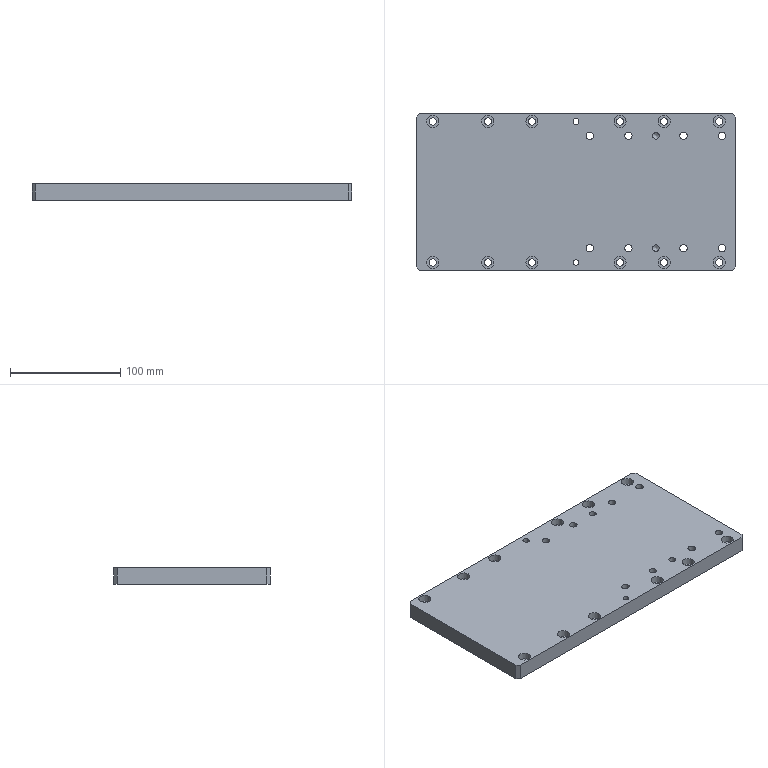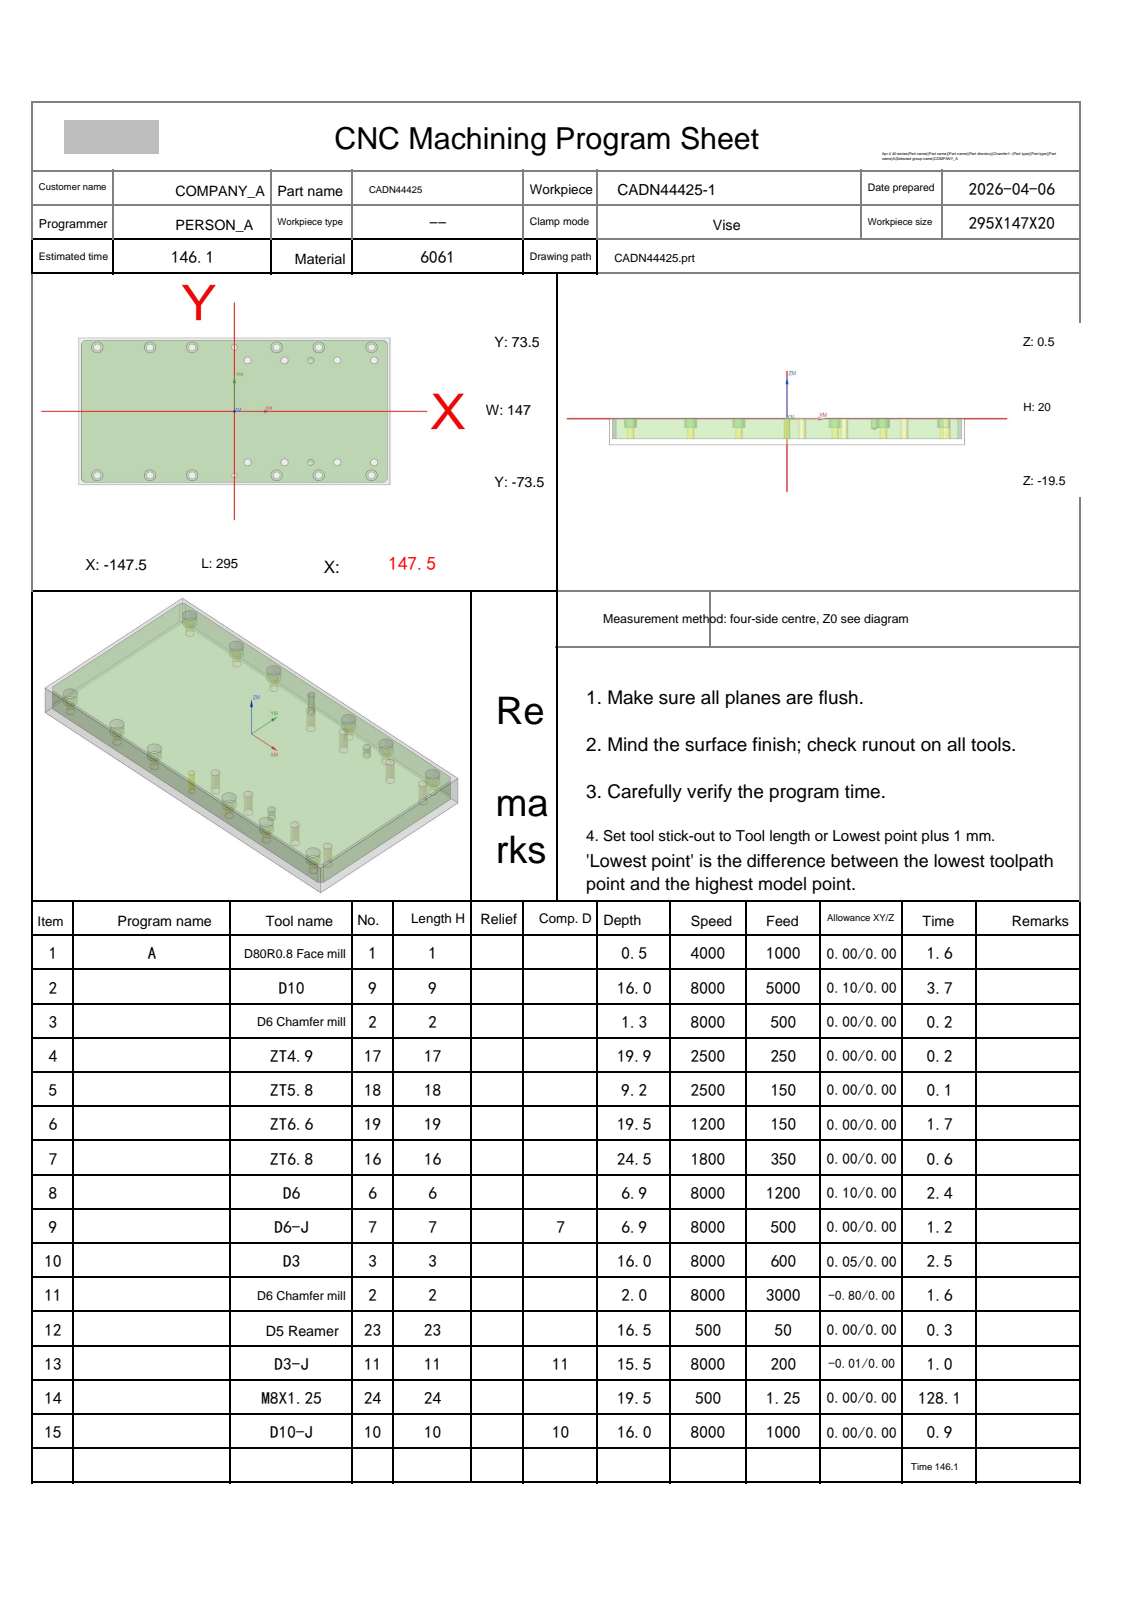NC program | NX | posted by the shop | part box 290 x 142 x 15 mm
Lines 1802 to 2582 of 2582:
N11 T02 M06
(D6 Chamfer mill  D=6. R=0. H=02 ce=0.00 di=0.00)
G00 G90 G54 X.25 Y-73.128 M03 S8000
G43 H02 Z20.
M08
Z2.099
G01 Z-1.5 F3000.
G03 X.33 Y-72.828 I-.52 J.3
X.03 Y-72.308 I-.6 J0.0
G01 X0.0 Y-72.3
X-142.
X-142.254 Y-72.275
X-142.497 Y-72.201
X-142.722 Y-72.081
X-142.919 Y-71.919
X-145.919 Y-68.919
X-146.081 Y-68.722
X-146.201 Y-68.497
X-146.275 Y-68.254
X-146.3 Y-68.
Y68.
X-146.275 Y68.254
X-146.201 Y68.497
X-146.081 Y68.722
X-145.919 Y68.919
X-142.919 Y71.919
X-142.722 Y72.081
X-142.497 Y72.201
X-142.254 Y72.275
X-142. Y72.3
X142.
X142.254 Y72.275
X142.497 Y72.201
X142.722 Y72.081
X142.919 Y71.919
X145.919 Y68.919
X146.081 Y68.722
X146.201 Y68.497
X146.275 Y68.254
X146.3 Y68.
Y-68.
X146.275 Y-68.254
X146.201 Y-68.497
X146.081 Y-68.722
X145.919 Y-68.919
X142.919 Y-71.919
X142.722 Y-72.081
X142.497 Y-72.201
X142.254 Y-72.275
X142. Y-72.3
X0.0
X-.03 Y-72.308
G03 X-.33 Y-72.828 I.3 J-.52
X-.25 Y-73.128 I.6 J0.0
G01 Z2.099
G00 Z20.
X-.372 Y64.25
Z2.099
G01 Z-1.5
G03 X-.672 Y64.33 I-.3 J-.52
X-1.192 Y64.03 I0.0 J-.6
G01 X-1.2 Y64.
Y63.5
G03 X0.0 Y62.3 I1.2 J0.0
X1.2 Y63.5 I0.0 J1.2
G01 Y64.5
G03 X0.0 Y65.7 I-1.2 J0.0
X-1.2 Y64.5 I0.0 J-1.2
G01 Y64.
X-1.192 Y63.97
G03 X-.672 Y63.67 I.52 J.3
X-.372 Y63.75 I0.0 J.6
G01 Z2.099
G00 Z20.
G00 G90 X-.157 Y-63.216 M03 S8000
Z20.
Z-.5
G01 Z-1. F500.
X-.3 Y-62.5
G03 X-1.8 Y-64. I0.0 J-1.5
X0.0 Y-65.8 I1.8 J0.0
X1.8 Y-64. I0.0 J1.8
X0.0 Y-62.2 I-1.8 J0.0
X-1.8 Y-64. I0.0 J-1.8
X-.3 Y-65.5 I1.5 J0.0
G01 X-.157 Y-64.784
Z-.5
G00 Z20.
G00 G90 X71.888 Y52.147 M03 S8000
Z20.
Z-.5
G01 Z-1. F500.
X71.7 Y52.5
G03 X70.2 Y51. I0.0 J-1.5
X72.5 Y48.7 I2.3 J0.0
X74.8 Y51. I0.0 J2.3
X72.5 Y53.3 I-2.3 J0.0
X70.2 Y51. I0.0 J-2.3
X71.7 Y49.5 I1.5 J0.0
G01 X71.888 Y49.853
Z-.5
G00 Z20.
Y-49.853
Z-.5
G01 Z-1.
X71.7 Y-49.5
G03 X70.2 Y-51. I0.0 J-1.5
X72.5 Y-53.3 I2.3 J0.0
X74.8 Y-51. I0.0 J2.3
X72.5 Y-48.7 I-2.3 J0.0
X70.2 Y-51. I0.0 J-2.3
X71.7 Y-52.5 I1.5 J0.0
G01 X71.888 Y-52.147
Z-.5
G00 Z20.
G00 G90 X131.334 Y52.5 M03 S8000
Z20.
Z-.8
G01 Z-1.3 F600.
X131.1
G03 X129.6 Y51. I0.0 J-1.5
X132.5 Y48.1 I2.9 J0.0
X135.4 Y51. I0.0 J2.9
X132.5 Y53.9 I-2.9 J0.0
X129.6 Y51. I0.0 J-2.9
X131.1 Y49.5 I1.5 J0.0
G01 X131.334
Z-.8
G00 Z20.
X96.334 Y52.5
Z-.8
G01 Z-1.3
X96.1
G03 X94.6 Y51. I0.0 J-1.5
X97.5 Y48.1 I2.9 J0.0
X100.4 Y51. I0.0 J2.9
X97.5 Y53.9 I-2.9 J0.0
X94.6 Y51. I0.0 J-2.9
X96.1 Y49.5 I1.5 J0.0
G01 X96.334
Z-.8
G00 Z20.
X46.334 Y52.5
Z-.8
G01 Z-1.3
X46.1
G03 X44.6 Y51. I0.0 J-1.5
X47.5 Y48.1 I2.9 J0.0
X50.4 Y51. I0.0 J2.9
X47.5 Y53.9 I-2.9 J0.0
X44.6 Y51. I0.0 J-2.9
X46.1 Y49.5 I1.5 J0.0
G01 X46.334
Z-.8
G00 Z20.
X11.334 Y52.5
Z-.8
G01 Z-1.3
X11.1
G03 X9.6 Y51. I0.0 J-1.5
X12.5 Y48.1 I2.9 J0.0
X15.4 Y51. I0.0 J2.9
X12.5 Y53.9 I-2.9 J0.0
X9.6 Y51. I0.0 J-2.9
X11.1 Y49.5 I1.5 J0.0
G01 X11.334
Z-.8
G00 Z20.
Y-49.5
Z-.8
G01 Z-1.3
X11.1
G03 X9.6 Y-51. I0.0 J-1.5
X12.5 Y-53.9 I2.9 J0.0
X15.4 Y-51. I0.0 J2.9
X12.5 Y-48.1 I-2.9 J0.0
X9.6 Y-51. I0.0 J-2.9
X11.1 Y-52.5 I1.5 J0.0
G01 X11.334
Z-.8
G00 Z20.
X46.334 Y-49.5
Z-.8
G01 Z-1.3
X46.1
G03 X44.6 Y-51. I0.0 J-1.5
X47.5 Y-53.9 I2.9 J0.0
X50.4 Y-51. I0.0 J2.9
X47.5 Y-48.1 I-2.9 J0.0
X44.6 Y-51. I0.0 J-2.9
X46.1 Y-52.5 I1.5 J0.0
G01 X46.334
Z-.8
G00 Z20.
X96.334 Y-49.5
Z-.8
G01 Z-1.3
X96.1
G03 X94.6 Y-51. I0.0 J-1.5
X97.5 Y-53.9 I2.9 J0.0
X100.4 Y-51. I0.0 J2.9
X97.5 Y-48.1 I-2.9 J0.0
X94.6 Y-51. I0.0 J-2.9
X96.1 Y-52.5 I1.5 J0.0
G01 X96.334
Z-.8
G00 Z20.
X131.334 Y-49.5
Z-.8
G01 Z-1.3
X131.1
G03 X129.6 Y-51. I0.0 J-1.5
X132.5 Y-53.9 I2.9 J0.0
X135.4 Y-51. I0.0 J2.9
X132.5 Y-48.1 I-2.9 J0.0
X129.6 Y-51. I0.0 J-2.9
X131.1 Y-52.5 I1.5 J0.0
G01 X131.334
Z-.8
G00 Z20.
G00 G90 X127.991 Y-68.357 M03 S8000
Z20.
Z2.5
G01 X128.166 Y-68.439 Z2.43 F800.
X128.601 Y-68.595 Z2.261
X129.05 Y-68.708 Z2.093
X129.507 Y-68.778 Z1.925
X129.969 Y-68.803 Z1.756
X130.431 Y-68.784 Z1.588
X130.89 Y-68.72 Z1.419
X131.34 Y-68.612 Z1.251
X131.777 Y-68.462 Z1.083
X132.198 Y-68.27 Z.914
X132.599 Y-68.039 Z.746
X132.976 Y-67.77 Z.577
X133.325 Y-67.466 Z.409
X133.643 Y-67.13 Z.241
X133.927 Y-66.765 Z.072
X134.175 Y-66.375 Z-.096
X134.384 Y-65.962 Z-.265
X134.552 Y-65.531 Z-.433
X134.679 Y-65.086 Z-.601
X134.761 Y-64.631 Z-.77
X134.8 Y-64.17 Z-.938
Y-64. Z-1.
G03 X130. Y-59.2 I-4.8 J0.0
X125.2 Y-64. I0.0 J-4.8
X130. Y-68.8 I4.8 J0.0
X134.8 Y-64. I0.0 J4.8
X134.774 Y-63.501 I-4.8 J0.0
G01 Z1.5
G00 Z20.
X77.991 Y-68.357
Z2.5
G01 X78.166 Y-68.439 Z2.43
X78.601 Y-68.595 Z2.261
X79.05 Y-68.708 Z2.093
X79.507 Y-68.778 Z1.925
X79.969 Y-68.803 Z1.756
X80.431 Y-68.784 Z1.588
X80.89 Y-68.72 Z1.419
X81.34 Y-68.612 Z1.251
X81.777 Y-68.462 Z1.083
X82.198 Y-68.27 Z.914
X82.599 Y-68.039 Z.746
X82.976 Y-67.77 Z.577
X83.325 Y-67.466 Z.409
X83.643 Y-67.13 Z.241
X83.927 Y-66.765 Z.072
X84.175 Y-66.375 Z-.096
X84.384 Y-65.962 Z-.265
X84.552 Y-65.531 Z-.433
X84.679 Y-65.086 Z-.601
X84.761 Y-64.631 Z-.77
X84.8 Y-64.17 Z-.938
Y-64. Z-1.
G03 X80. Y-59.2 I-4.8 J0.0
X75.2 Y-64. I0.0 J-4.8
X80. Y-68.8 I4.8 J0.0
X84.8 Y-64. I0.0 J4.8
X84.774 Y-63.501 I-4.8 J0.0
G01 Z1.5
G00 Z20.
X37.991 Y-68.357
Z2.5
G01 X38.166 Y-68.439 Z2.43
X38.601 Y-68.595 Z2.261
X39.05 Y-68.708 Z2.093
X39.507 Y-68.778 Z1.925
X39.969 Y-68.803 Z1.756
X40.431 Y-68.784 Z1.588
X40.89 Y-68.72 Z1.419
X41.34 Y-68.612 Z1.251
X41.777 Y-68.462 Z1.083
X42.198 Y-68.27 Z.914
X42.599 Y-68.039 Z.746
X42.976 Y-67.77 Z.577
X43.325 Y-67.466 Z.409
X43.643 Y-67.13 Z.241
X43.927 Y-66.765 Z.072
X44.175 Y-66.375 Z-.096
X44.384 Y-65.962 Z-.265
X44.552 Y-65.531 Z-.433
X44.679 Y-65.086 Z-.601
X44.761 Y-64.631 Z-.77
X44.8 Y-64.17 Z-.938
Y-64. Z-1.
G03 X40. Y-59.2 I-4.8 J0.0
X35.2 Y-64. I0.0 J-4.8
X40. Y-68.8 I4.8 J0.0
X44.8 Y-64. I0.0 J4.8
X44.774 Y-63.501 I-4.8 J0.0
G01 Z1.5
G00 Z20.
X-42.009 Y-68.357
Z2.5
G01 X-41.834 Y-68.439 Z2.43
X-41.399 Y-68.595 Z2.261
X-40.95 Y-68.708 Z2.093
X-40.493 Y-68.778 Z1.925
X-40.031 Y-68.803 Z1.756
X-39.569 Y-68.784 Z1.588
X-39.11 Y-68.72 Z1.419
X-38.66 Y-68.612 Z1.251
X-38.223 Y-68.462 Z1.083
X-37.802 Y-68.27 Z.914
X-37.401 Y-68.039 Z.746
X-37.024 Y-67.77 Z.577
X-36.675 Y-67.466 Z.409
X-36.357 Y-67.13 Z.241
X-36.073 Y-66.765 Z.072
X-35.825 Y-66.375 Z-.096
X-35.616 Y-65.962 Z-.265
X-35.448 Y-65.531 Z-.433
X-35.321 Y-65.086 Z-.601
X-35.239 Y-64.631 Z-.77
X-35.2 Y-64.17 Z-.938
Y-64. Z-1.
G03 X-40. Y-59.2 I-4.8 J0.0
X-44.8 Y-64. I0.0 J-4.8
X-40. Y-68.8 I4.8 J0.0
X-35.2 Y-64. I0.0 J4.8
X-35.226 Y-63.501 I-4.8 J0.0
G01 Z1.5
G00 Z20.
X-82.009 Y-68.357
Z2.5
G01 X-81.834 Y-68.439 Z2.43
X-81.399 Y-68.595 Z2.261
X-80.95 Y-68.708 Z2.093
X-80.493 Y-68.778 Z1.925
X-80.031 Y-68.803 Z1.756
X-79.569 Y-68.784 Z1.588
X-79.11 Y-68.72 Z1.419
X-78.66 Y-68.612 Z1.251
X-78.223 Y-68.462 Z1.083
X-77.802 Y-68.27 Z.914
X-77.401 Y-68.039 Z.746
X-77.024 Y-67.77 Z.577
X-76.675 Y-67.466 Z.409
X-76.357 Y-67.13 Z.241
X-76.073 Y-66.765 Z.072
X-75.825 Y-66.375 Z-.096
X-75.616 Y-65.962 Z-.265
X-75.448 Y-65.531 Z-.433
X-75.321 Y-65.086 Z-.601
X-75.239 Y-64.631 Z-.77
X-75.2 Y-64.17 Z-.938
Y-64. Z-1.
G03 X-80. Y-59.2 I-4.8 J0.0
X-84.8 Y-64. I0.0 J-4.8
X-80. Y-68.8 I4.8 J0.0
X-75.2 Y-64. I0.0 J4.8
X-75.226 Y-63.501 I-4.8 J0.0
G01 Z1.5
G00 Z20.
X-132.009 Y-68.357
Z2.5
G01 X-131.834 Y-68.439 Z2.43
X-131.399 Y-68.595 Z2.261
X-130.95 Y-68.708 Z2.093
X-130.493 Y-68.778 Z1.925
X-130.031 Y-68.803 Z1.756
X-129.569 Y-68.784 Z1.588
X-129.11 Y-68.72 Z1.419
X-128.66 Y-68.612 Z1.251
X-128.223 Y-68.462 Z1.083
X-127.802 Y-68.27 Z.914
X-127.401 Y-68.039 Z.746
X-127.024 Y-67.77 Z.577
X-126.675 Y-67.466 Z.409
X-126.357 Y-67.13 Z.241
X-126.073 Y-66.765 Z.072
X-125.825 Y-66.375 Z-.096
X-125.616 Y-65.962 Z-.265
X-125.448 Y-65.531 Z-.433
X-125.321 Y-65.086 Z-.601
X-125.239 Y-64.631 Z-.77
X-125.2 Y-64.17 Z-.938
Y-64. Z-1.
G03 X-130. Y-59.2 I-4.8 J0.0
X-134.8 Y-64. I0.0 J-4.8
X-130. Y-68.8 I4.8 J0.0
X-125.2 Y-64. I0.0 J4.8
X-125.226 Y-63.501 I-4.8 J0.0
G01 Z1.5
G00 Z20.
X-132.009 Y59.643
Z2.5
G01 X-131.834 Y59.561 Z2.43
X-131.399 Y59.405 Z2.261
X-130.95 Y59.292 Z2.093
X-130.493 Y59.222 Z1.925
X-130.031 Y59.197 Z1.756
X-129.569 Y59.216 Z1.588
X-129.11 Y59.28 Z1.419
X-128.66 Y59.388 Z1.251
X-128.223 Y59.538 Z1.083
X-127.802 Y59.73 Z.914
X-127.401 Y59.961 Z.746
X-127.024 Y60.23 Z.577
X-126.675 Y60.534 Z.409
X-126.357 Y60.87 Z.241
X-126.073 Y61.235 Z.072
X-125.825 Y61.625 Z-.096
X-125.616 Y62.038 Z-.265
X-125.448 Y62.469 Z-.433
X-125.321 Y62.914 Z-.601
X-125.239 Y63.369 Z-.77
X-125.2 Y63.83 Z-.938
Y64. Z-1.
G03 X-130. Y68.8 I-4.8 J0.0
X-134.8 Y64. I0.0 J-4.8
X-130. Y59.2 I4.8 J0.0
X-125.2 Y64. I0.0 J4.8
X-125.226 Y64.499 I-4.8 J0.0
G01 Z1.5
G00 Z20.
X-82.009 Y59.643
Z2.5
G01 X-81.834 Y59.561 Z2.43
X-81.399 Y59.405 Z2.261
X-80.95 Y59.292 Z2.093
X-80.493 Y59.222 Z1.925
X-80.031 Y59.197 Z1.756
X-79.569 Y59.216 Z1.588
X-79.11 Y59.28 Z1.419
X-78.66 Y59.388 Z1.251
X-78.223 Y59.538 Z1.083
X-77.802 Y59.73 Z.914
X-77.401 Y59.961 Z.746
X-77.024 Y60.23 Z.577
X-76.675 Y60.534 Z.409
X-76.357 Y60.87 Z.241
X-76.073 Y61.235 Z.072
X-75.825 Y61.625 Z-.096
X-75.616 Y62.038 Z-.265
X-75.448 Y62.469 Z-.433
X-75.321 Y62.914 Z-.601
X-75.239 Y63.369 Z-.77
X-75.2 Y63.83 Z-.938
Y64. Z-1.
G03 X-80. Y68.8 I-4.8 J0.0
X-84.8 Y64. I0.0 J-4.8
X-80. Y59.2 I4.8 J0.0
X-75.2 Y64. I0.0 J4.8
X-75.226 Y64.499 I-4.8 J0.0
G01 Z1.5
G00 Z20.
X-42.009 Y59.643
Z2.5
G01 X-41.834 Y59.561 Z2.43
X-41.399 Y59.405 Z2.261
X-40.95 Y59.292 Z2.093
X-40.493 Y59.222 Z1.925
X-40.031 Y59.197 Z1.756
X-39.569 Y59.216 Z1.588
X-39.11 Y59.28 Z1.419
X-38.66 Y59.388 Z1.251
X-38.223 Y59.538 Z1.083
X-37.802 Y59.73 Z.914
X-37.401 Y59.961 Z.746
X-37.024 Y60.23 Z.577
X-36.675 Y60.534 Z.409
X-36.357 Y60.87 Z.241
X-36.073 Y61.235 Z.072
X-35.825 Y61.625 Z-.096
X-35.616 Y62.038 Z-.265
X-35.448 Y62.469 Z-.433
X-35.321 Y62.914 Z-.601
X-35.239 Y63.369 Z-.77
X-35.2 Y63.83 Z-.938
Y64. Z-1.
G03 X-40. Y68.8 I-4.8 J0.0
X-44.8 Y64. I0.0 J-4.8
X-40. Y59.2 I4.8 J0.0
X-35.2 Y64. I0.0 J4.8
X-35.226 Y64.499 I-4.8 J0.0
G01 Z1.5
G00 Z20.
X37.991 Y59.643
Z2.5
G01 X38.166 Y59.561 Z2.43
X38.601 Y59.405 Z2.261
X39.05 Y59.292 Z2.093
X39.507 Y59.222 Z1.925
X39.969 Y59.197 Z1.756
X40.431 Y59.216 Z1.588
X40.89 Y59.28 Z1.419
X41.34 Y59.388 Z1.251
X41.777 Y59.538 Z1.083
X42.198 Y59.73 Z.914
X42.599 Y59.961 Z.746
X42.976 Y60.23 Z.577
X43.325 Y60.534 Z.409
X43.643 Y60.87 Z.241
X43.927 Y61.235 Z.072
X44.175 Y61.625 Z-.096
X44.384 Y62.038 Z-.265
X44.552 Y62.469 Z-.433
X44.679 Y62.914 Z-.601
X44.761 Y63.369 Z-.77
X44.8 Y63.83 Z-.938
Y64. Z-1.
G03 X40. Y68.8 I-4.8 J0.0
X35.2 Y64. I0.0 J-4.8
X40. Y59.2 I4.8 J0.0
X44.8 Y64. I0.0 J4.8
X44.774 Y64.499 I-4.8 J0.0
G01 Z1.5
G00 Z20.
X77.991 Y59.643
Z2.5
G01 X78.166 Y59.561 Z2.43
X78.601 Y59.405 Z2.261
X79.05 Y59.292 Z2.093
X79.507 Y59.222 Z1.925
X79.969 Y59.197 Z1.756
X80.431 Y59.216 Z1.588
X80.89 Y59.28 Z1.419
X81.34 Y59.388 Z1.251
X81.777 Y59.538 Z1.083
X82.198 Y59.73 Z.914
X82.599 Y59.961 Z.746
X82.976 Y60.23 Z.577
X83.325 Y60.534 Z.409
X83.643 Y60.87 Z.241
X83.927 Y61.235 Z.072
X84.175 Y61.625 Z-.096
X84.384 Y62.038 Z-.265
X84.552 Y62.469 Z-.433
X84.679 Y62.914 Z-.601
X84.761 Y63.369 Z-.77
X84.8 Y63.83 Z-.938
Y64. Z-1.
G03 X80. Y68.8 I-4.8 J0.0
X75.2 Y64. I0.0 J-4.8
X80. Y59.2 I4.8 J0.0
X84.8 Y64. I0.0 J4.8
X84.774 Y64.499 I-4.8 J0.0
G01 Z1.5
G00 Z20.
X127.991 Y59.643
Z2.5
G01 X128.166 Y59.561 Z2.43
X128.601 Y59.405 Z2.261
X129.05 Y59.292 Z2.093
X129.507 Y59.222 Z1.925
X129.969 Y59.197 Z1.756
X130.431 Y59.216 Z1.588
X130.89 Y59.28 Z1.419
X131.34 Y59.388 Z1.251
X131.777 Y59.538 Z1.083
X132.198 Y59.73 Z.914
X132.599 Y59.961 Z.746
X132.976 Y60.23 Z.577
X133.325 Y60.534 Z.409
X133.643 Y60.87 Z.241
X133.927 Y61.235 Z.072
X134.175 Y61.625 Z-.096
X134.384 Y62.038 Z-.265
X134.552 Y62.469 Z-.433
X134.679 Y62.914 Z-.601
X134.761 Y63.369 Z-.77
X134.8 Y63.83 Z-.938
Y64. Z-1.
G03 X130. Y68.8 I-4.8 J0.0
X125.2 Y64. I0.0 J-4.8
X130. Y59.2 I4.8 J0.0
X134.8 Y64. I0.0 J4.8
X134.774 Y64.499 I-4.8 J0.0
G01 Z1.5
G00 Z20.
G91 G28 Z0.0
M05
M09
G91 G28 Z0.0
M01
N12 T23 M06
(D5 Reamer D=5. DR_a=180 H=23)
G00 G90 G54 X0.0 Y-64. M03 S500
G43 H23 Z20.
M08
G98 G81 X0.0 Y-64. Z-16. R1. F50.
G80
G00 Z20.
G91 G28 Z0.0
M05
M09
G91 G28 Z0.0
M01
N13 T11 M06
(D3-J  D=3. R=0. H=11 ce=-0.01 di=0.00)
G00 G90 G54 X72.5 Y51. M03 S8000
G43 H11 Z20.
M08
Z.5
G41 D11
G01 X72.552 Y50.807 F200.
G03 X73.268 Y50.258 I.716 J.193
X74.01 Y51. I0.0 J.742
X74.01 Y51. Z-.5 I-1.51 J0.0
X74.01 Y51. Z-1.5 I-1.51 J0.0
X74.01 Y51. Z-2.5 I-1.51 J0.0
X74.01 Y51. Z-3.5 I-1.51 J0.0
X74.01 Y51. Z-4.5 I-1.51 J0.0
X74.01 Y51. Z-5.5 I-1.51 J0.0
X74.01 Y51. Z-6.5 I-1.51 J0.0
X70.99 Y51. Z-7. I-1.51 J0.0
X72.5 Y49.49 I1.51 J0.0
X74.01 Y51. I0.0 J1.51
X72.5 Y52.51 I-1.51 J0.0
X70.99 Y51. I0.0 J-1.51
X71.732 Y50.258 I.742 J0.0
X72.448 Y50.807 I0.0 J.742
G01 G40 X72.5 Y51.
G00 Z20.
Y-51.
Z.5
G41 D11
G01 X72.552 Y-51.193
G03 X73.268 Y-51.742 I.716 J.193
X74.01 Y-51. I0.0 J.742
X74.01 Y-51. Z-.5 I-1.51 J0.0
X74.01 Y-51. Z-1.5 I-1.51 J0.0
X74.01 Y-51. Z-2.5 I-1.51 J0.0
X74.01 Y-51. Z-3.5 I-1.51 J0.0
X74.01 Y-51. Z-4.5 I-1.51 J0.0
X74.01 Y-51. Z-5.5 I-1.51 J0.0
X74.01 Y-51. Z-6.5 I-1.51 J0.0
X70.99 Y-51. Z-7. I-1.51 J0.0
X72.5 Y-52.51 I1.51 J0.0
X74.01 Y-51. I0.0 J1.51
X72.5 Y-49.49 I-1.51 J0.0
X70.99 Y-51. I0.0 J-1.51
X71.732 Y-51.742 I.742 J0.0
X72.448 Y-51.193 I0.0 J.742
G01 G40 X72.5 Y-51.
G00 Z20.
G00 G90 X.76 Y63.8 M03 S6000
Z20.
Z-4.5
G01 Z-5. F200.
G41 D11
X.81
G03 X1.01 Y64. I0.0 J.2
G01 Y64.5
G03 X0.0 Y65.51 I-1.01 J0.0
X-1.01 Y64.5 I0.0 J-1.01
G01 Y63.5
G03 X0.0 Y62.49 I1.01 J0.0
X1.01 Y63.5 I0.0 J1.01
G01 Y64.
Y64.5
G03 X.81 Y64.7 I-.2 J0.0
G01 X.785
G40 X.735
Z-4.5
G00 Z.5
X.76 Y63.8
Z-9.5
G01 Z-10.
G41 D11
X.81
G03 X1.01 Y64. I0.0 J.2
G01 Y64.5
G03 X0.0 Y65.51 I-1.01 J0.0
X-1.01 Y64.5 I0.0 J-1.01
G01 Y63.5
G03 X0.0 Y62.49 I1.01 J0.0
X1.01 Y63.5 I0.0 J1.01
G01 Y64.
Y64.5
G03 X.81 Y64.7 I-.2 J0.0
G01 X.785
G40 X.735
Z-9.5
G00 Z-4.5
X.76 Y63.8
Z-14.5
G01 Z-15.
G41 D11
X.81
G03 X1.01 Y64. I0.0 J.2
G01 Y64.5
G03 X0.0 Y65.51 I-1.01 J0.0
X-1.01 Y64.5 I0.0 J-1.01
G01 Y63.5
G03 X0.0 Y62.49 I1.01 J0.0
X1.01 Y63.5 I0.0 J1.01
G01 Y64.
Y64.5
G03 X.81 Y64.7 I-.2 J0.0
G01 X.785
G40 X.735
Z-14.5
G00 Z20.
G91 G28 Z0.0
M05
M09
G91 G28 Z0.0
M01
N14 T24 M06
(M8X1.25 D=6.8 DR_a=180 H=24)
G00 G90 G54 X132.5 Y-51. M03 S500
G43 H24 Z20.
M08
G95
G98 G84 X132.5 Y-51. Z-19. R1. F1.25 Q4.
X97.5
X47.5
X12.5
Y51.
X47.5
X97.5
X132.5
G80
G94
G00 Z20.
G91 G28 Z0.0
M05
M09
G91 G28 Z0.0
M01
N15 T10 M06
(D10-J  D=10. R=0. H=10 ce=0.00 di=0.00)
G00 G90 G54 X143.013 Y-77.116 M03 S8000
G43 H10 Z20.
M08
Z-15.
G01 Z-15.5 F1000.
G41 D10
X142.997 Y-76.917
G03 X142. Y-76. I-.997 J-.083
G01 X-142.
G02 X-145.536 Y-74.536 I0.0 J5.
G01 X-148.536 Y-71.536
G02 X-150. Y-68. I3.536 J3.536
G01 Y68.
G02 X-148.536 Y71.536 I5. J0.0
G01 X-145.536 Y74.536
G02 X-142. Y76. I3.536 J-3.536
G01 X142.
G02 X145.536 Y74.536 I0.0 J-5.
G01 X148.536 Y71.536
G02 X150. Y68. I-3.536 J-3.536
G01 Y-68.
G02 X148.536 Y-71.536 I-5. J0.0
G01 X145.536 Y-74.536
G02 X142. Y-76. I-3.536 J3.536
G01 X141.5
G03 X140.5 Y-77. I0.0 J-1.
G01 G40 Y-77.2
Z-15.
G00 Z20.
M05
M09
G91 G28 Z0.0
G91 G28 Y0.0
M30
%